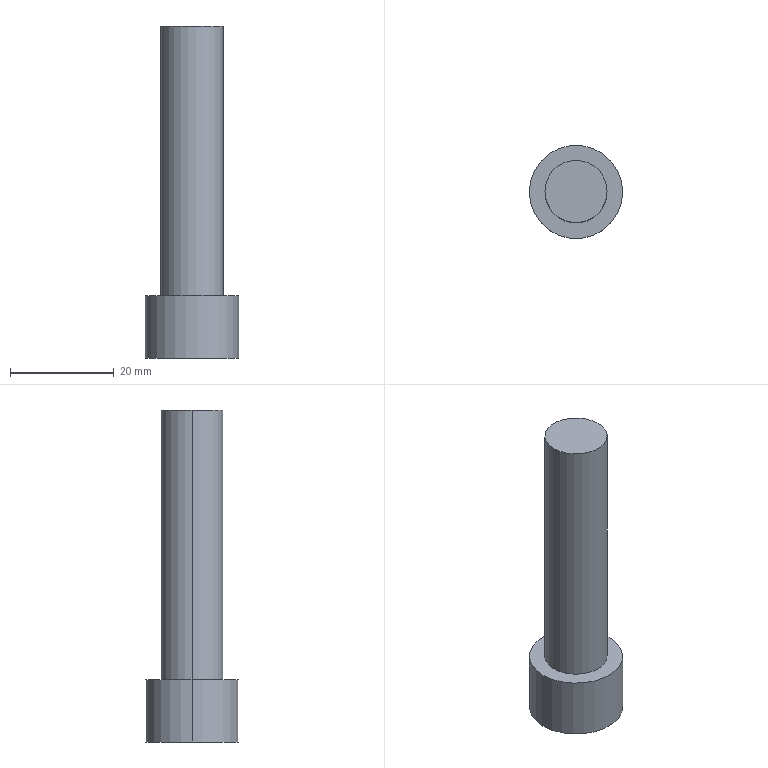Part | Creo | 1 solid | 14 faces | box 18 x 18 x 64 mm | volume 8415 mm3 | plane 10 | cylinder 4 | commonest cylinder face diameters 12 x2 18 x2
STEP:
#1=CARTESIAN_POINT('',(189.,0.,-294.5));
#2=VERTEX_POINT('',#1);
#3=CARTESIAN_POINT('',(171.,0.,-294.5));
#4=VERTEX_POINT('',#3);
#5=CARTESIAN_POINT('',(180.,0.,-294.5));
#6=DIRECTION('',(0.,0.,-1.));
#7=DIRECTION('',(1.,0.,0.));
#8=AXIS2_PLACEMENT_3D('',#5,#6,#7);
#9=CIRCLE('',#8,9.);
#10=EDGE_CURVE('',#2,#4,#9,.T.);
#11=ORIENTED_EDGE('',*,*,#10,.F.);
#12=CARTESIAN_POINT('',(180.,0.,-294.5));
#13=DIRECTION('',(0.,0.,-1.));
#14=DIRECTION('',(-1.,0.,0.));
#15=AXIS2_PLACEMENT_3D('',#12,#13,#14);
#16=CIRCLE('',#15,9.);
#17=EDGE_CURVE('',#4,#2,#16,.T.);
#18=ORIENTED_EDGE('',*,*,#17,.F.);
#19=EDGE_LOOP('',(#11,#18));
#20=FACE_OUTER_BOUND('',#19,.F.);
#21=CARTESIAN_POINT('',(175.,-2.887,-294.5));
#22=VERTEX_POINT('',#21);
#23=CARTESIAN_POINT('',(180.,-5.774,-294.5));
#24=VERTEX_POINT('',#23);
#25=CARTESIAN_POINT('',(175.,-2.887,-294.5));
#26=DIRECTION('',(0.866,-0.5,0.));
#27=VECTOR('',#26,5.774);
#28=LINE('',#25,#27);
#29=EDGE_CURVE('',#22,#24,#28,.T.);
#30=ORIENTED_EDGE('',*,*,#29,.F.);
#31=CARTESIAN_POINT('',(175.,2.887,-294.5));
#32=VERTEX_POINT('',#31);
#33=CARTESIAN_POINT('',(175.,-2.887,-294.5));
#34=DIRECTION('',(0.,1.,0.));
#35=VECTOR('',#34,5.774);
#36=LINE('',#33,#35);
#37=EDGE_CURVE('',#22,#32,#36,.T.);
#38=ORIENTED_EDGE('',*,*,#37,.T.);
#39=CARTESIAN_POINT('',(180.,5.774,-294.5));
#40=VERTEX_POINT('',#39);
#41=CARTESIAN_POINT('',(180.,5.774,-294.5));
#42=DIRECTION('',(-0.866,-0.5,0.));
#43=VECTOR('',#42,5.774);
#44=LINE('',#41,#43);
#45=EDGE_CURVE('',#40,#32,#44,.T.);
#46=ORIENTED_EDGE('',*,*,#45,.F.);
#47=CARTESIAN_POINT('',(185.,2.887,-294.5));
#48=VERTEX_POINT('',#47);
#49=CARTESIAN_POINT('',(185.,2.887,-294.5));
#50=DIRECTION('',(-0.866,0.5,0.));
#51=VECTOR('',#50,5.774);
#52=LINE('',#49,#51);
#53=EDGE_CURVE('',#48,#40,#52,.T.);
#54=ORIENTED_EDGE('',*,*,#53,.F.);
#55=CARTESIAN_POINT('',(185.,-2.887,-294.5));
#56=VERTEX_POINT('',#55);
#57=CARTESIAN_POINT('',(185.,2.887,-294.5));
#58=DIRECTION('',(0.,-1.,0.));
#59=VECTOR('',#58,5.774);
#60=LINE('',#57,#59);
#61=EDGE_CURVE('',#48,#56,#60,.T.);
#62=ORIENTED_EDGE('',*,*,#61,.T.);
#63=CARTESIAN_POINT('',(180.,-5.774,-294.5));
#64=DIRECTION('',(0.866,0.5,0.));
#65=VECTOR('',#64,5.774);
#66=LINE('',#63,#65);
#67=EDGE_CURVE('',#24,#56,#66,.T.);
#68=ORIENTED_EDGE('',*,*,#67,.F.);
#69=EDGE_LOOP('',(#30,#38,#46,#54,#62,#68));
#70=FACE_BOUND('',#69,.F.);
#71=CARTESIAN_POINT('',(180.,0.,-294.5));
#72=DIRECTION('',(0.,0.,-1.));
#73=DIRECTION('',(-1.,0.,0.));
#74=AXIS2_PLACEMENT_3D('',#71,#72,#73);
#75=PLANE('',#74);
#76=ADVANCED_FACE('',(#20,#70),#75,.T.);
#77=CARTESIAN_POINT('',(171.,0.,-282.5));
#78=VERTEX_POINT('',#77);
#79=CARTESIAN_POINT('',(189.,0.,-282.5));
#80=VERTEX_POINT('',#79);
#81=CARTESIAN_POINT('',(180.,0.,-282.5));
#82=DIRECTION('',(0.,0.,1.));
#83=DIRECTION('',(-1.,0.,0.));
#84=AXIS2_PLACEMENT_3D('',#81,#82,#83);
#85=CIRCLE('',#84,9.);
#86=EDGE_CURVE('',#78,#80,#85,.T.);
#87=ORIENTED_EDGE('',*,*,#86,.T.);
#88=CARTESIAN_POINT('',(189.,0.,-294.5));
#89=DIRECTION('',(0.,0.,1.));
#90=VECTOR('',#89,12.);
#91=LINE('',#88,#90);
#92=EDGE_CURVE('',#2,#80,#91,.T.);
#93=ORIENTED_EDGE('',*,*,#92,.F.);
#94=ORIENTED_EDGE('',*,*,#10,.T.);
#95=CARTESIAN_POINT('',(171.,0.,-294.5));
#96=DIRECTION('',(0.,0.,1.));
#97=VECTOR('',#96,12.);
#98=LINE('',#95,#97);
#99=EDGE_CURVE('',#4,#78,#98,.T.);
#100=ORIENTED_EDGE('',*,*,#99,.T.);
#101=EDGE_LOOP('',(#87,#93,#94,#100));
#102=FACE_OUTER_BOUND('',#101,.F.);
#103=CARTESIAN_POINT('',(180.,0.,-294.5));
#104=DIRECTION('',(0.,0.,1.));
#105=DIRECTION('',(1.,0.,0.));
#106=AXIS2_PLACEMENT_3D('',#103,#104,#105);
#107=CYLINDRICAL_SURFACE('',#106,9.);
#108=ADVANCED_FACE('',(#102),#107,.T.);
#109=ORIENTED_EDGE('',*,*,#86,.F.);
#110=CARTESIAN_POINT('',(180.,0.,-282.5));
#111=DIRECTION('',(0.,0.,1.));
#112=DIRECTION('',(1.,0.,0.));
#113=AXIS2_PLACEMENT_3D('',#110,#111,#112);
#114=CIRCLE('',#113,9.);
#115=EDGE_CURVE('',#80,#78,#114,.T.);
#116=ORIENTED_EDGE('',*,*,#115,.F.);
#117=EDGE_LOOP('',(#109,#116));
#118=FACE_OUTER_BOUND('',#117,.F.);
#119=CARTESIAN_POINT('',(186.,0.,-282.5));
#120=VERTEX_POINT('',#119);
#121=CARTESIAN_POINT('',(174.,0.,-282.5));
#122=VERTEX_POINT('',#121);
#123=CARTESIAN_POINT('',(180.,0.,-282.5));
#124=DIRECTION('',(0.,0.,-1.));
#125=DIRECTION('',(1.,0.,0.));
#126=AXIS2_PLACEMENT_3D('',#123,#124,#125);
#127=CIRCLE('',#126,6.);
#128=EDGE_CURVE('',#120,#122,#127,.T.);
#129=ORIENTED_EDGE('',*,*,#128,.F.);
#130=CARTESIAN_POINT('',(180.,0.,-282.5));
#131=DIRECTION('',(0.,0.,-1.));
#132=DIRECTION('',(-1.,0.,0.));
#133=AXIS2_PLACEMENT_3D('',#130,#131,#132);
#134=CIRCLE('',#133,6.);
#135=EDGE_CURVE('',#122,#120,#134,.T.);
#136=ORIENTED_EDGE('',*,*,#135,.F.);
#137=EDGE_LOOP('',(#129,#136));
#138=FACE_BOUND('',#137,.F.);
#139=CARTESIAN_POINT('',(180.,0.,-282.5));
#140=DIRECTION('',(0.,0.,1.));
#141=DIRECTION('',(1.,0.,0.));
#142=AXIS2_PLACEMENT_3D('',#139,#140,#141);
#143=PLANE('',#142);
#144=ADVANCED_FACE('',(#118,#138),#143,.T.);
#145=ORIENTED_EDGE('',*,*,#128,.T.);
#146=CARTESIAN_POINT('',(174.,0.,-230.5));
#147=VERTEX_POINT('',#146);
#148=CARTESIAN_POINT('',(174.,0.,-282.5));
#149=DIRECTION('',(0.,0.,1.));
#150=VECTOR('',#149,52.);
#151=LINE('',#148,#150);
#152=EDGE_CURVE('',#122,#147,#151,.T.);
#153=ORIENTED_EDGE('',*,*,#152,.T.);
#154=CARTESIAN_POINT('',(186.,0.,-230.5));
#155=VERTEX_POINT('',#154);
#156=CARTESIAN_POINT('',(180.,0.,-230.5));
#157=DIRECTION('',(0.,0.,1.));
#158=DIRECTION('',(-1.,0.,0.));
#159=AXIS2_PLACEMENT_3D('',#156,#157,#158);
#160=CIRCLE('',#159,6.);
#161=EDGE_CURVE('',#147,#155,#160,.T.);
#162=ORIENTED_EDGE('',*,*,#161,.T.);
#163=CARTESIAN_POINT('',(186.,0.,-282.5));
#164=DIRECTION('',(0.,0.,1.));
#165=VECTOR('',#164,52.);
#166=LINE('',#163,#165);
#167=EDGE_CURVE('',#120,#155,#166,.T.);
#168=ORIENTED_EDGE('',*,*,#167,.F.);
#169=EDGE_LOOP('',(#145,#153,#162,#168));
#170=FACE_OUTER_BOUND('',#169,.F.);
#171=CARTESIAN_POINT('',(180.,0.,-284.5));
#172=DIRECTION('',(0.,0.,1.));
#173=DIRECTION('',(1.,0.,0.));
#174=AXIS2_PLACEMENT_3D('',#171,#172,#173);
#175=CYLINDRICAL_SURFACE('',#174,6.);
#176=ADVANCED_FACE('',(#170),#175,.T.);
#177=ORIENTED_EDGE('',*,*,#135,.T.);
#178=ORIENTED_EDGE('',*,*,#167,.T.);
#179=CARTESIAN_POINT('',(180.,0.,-230.5));
#180=DIRECTION('',(0.,0.,1.));
#181=DIRECTION('',(1.,0.,0.));
#182=AXIS2_PLACEMENT_3D('',#179,#180,#181);
#183=CIRCLE('',#182,6.);
#184=EDGE_CURVE('',#155,#147,#183,.T.);
#185=ORIENTED_EDGE('',*,*,#184,.T.);
#186=ORIENTED_EDGE('',*,*,#152,.F.);
#187=EDGE_LOOP('',(#177,#178,#185,#186));
#188=FACE_OUTER_BOUND('',#187,.F.);
#189=CARTESIAN_POINT('',(180.,0.,-284.5));
#190=DIRECTION('',(0.,0.,1.));
#191=DIRECTION('',(1.,0.,0.));
#192=AXIS2_PLACEMENT_3D('',#189,#190,#191);
#193=CYLINDRICAL_SURFACE('',#192,6.);
#194=ADVANCED_FACE('',(#188),#193,.T.);
#195=ORIENTED_EDGE('',*,*,#161,.F.);
#196=ORIENTED_EDGE('',*,*,#184,.F.);
#197=EDGE_LOOP('',(#195,#196));
#198=FACE_OUTER_BOUND('',#197,.F.);
#199=CARTESIAN_POINT('',(180.,0.,-230.5));
#200=DIRECTION('',(0.,0.,1.));
#201=DIRECTION('',(1.,0.,0.));
#202=AXIS2_PLACEMENT_3D('',#199,#200,#201);
#203=PLANE('',#202);
#204=ADVANCED_FACE('',(#198),#203,.T.);
#205=ORIENTED_EDGE('',*,*,#115,.T.);
#206=ORIENTED_EDGE('',*,*,#99,.F.);
#207=ORIENTED_EDGE('',*,*,#17,.T.);
#208=ORIENTED_EDGE('',*,*,#92,.T.);
#209=EDGE_LOOP('',(#205,#206,#207,#208));
#210=FACE_OUTER_BOUND('',#209,.F.);
#211=CARTESIAN_POINT('',(180.,0.,-294.5));
#212=DIRECTION('',(0.,0.,1.));
#213=DIRECTION('',(1.,0.,0.));
#214=AXIS2_PLACEMENT_3D('',#211,#212,#213);
#215=CYLINDRICAL_SURFACE('',#214,9.);
#216=ADVANCED_FACE('',(#210),#215,.T.);
#217=CARTESIAN_POINT('',(180.,-5.774,-288.5));
#218=VERTEX_POINT('',#217);
#219=CARTESIAN_POINT('',(175.,-2.887,-288.5));
#220=VERTEX_POINT('',#219);
#221=CARTESIAN_POINT('',(180.,-5.774,-288.5));
#222=DIRECTION('',(-0.866,0.5,0.));
#223=VECTOR('',#222,5.774);
#224=LINE('',#221,#223);
#225=EDGE_CURVE('',#218,#220,#224,.T.);
#226=ORIENTED_EDGE('',*,*,#225,.T.);
#227=CARTESIAN_POINT('',(175.,-2.887,-288.5));
#228=DIRECTION('',(0.,0.,-1.));
#229=VECTOR('',#228,6.);
#230=LINE('',#227,#229);
#231=EDGE_CURVE('',#220,#22,#230,.T.);
#232=ORIENTED_EDGE('',*,*,#231,.T.);
#233=ORIENTED_EDGE('',*,*,#29,.T.);
#234=CARTESIAN_POINT('',(180.,-5.774,-288.5));
#235=DIRECTION('',(0.,0.,-1.));
#236=VECTOR('',#235,6.);
#237=LINE('',#234,#236);
#238=EDGE_CURVE('',#218,#24,#237,.T.);
#239=ORIENTED_EDGE('',*,*,#238,.F.);
#240=EDGE_LOOP('',(#226,#232,#233,#239));
#241=FACE_OUTER_BOUND('',#240,.F.);
#242=CARTESIAN_POINT('',(177.5,-4.33,-291.5));
#243=DIRECTION('',(-0.5,-0.866,0.));
#244=DIRECTION('',(0.866,-0.5,0.));
#245=AXIS2_PLACEMENT_3D('',#242,#243,#244);
#246=PLANE('',#245);
#247=ADVANCED_FACE('',(#241),#246,.F.);
#248=CARTESIAN_POINT('',(175.,2.887,-288.5));
#249=VERTEX_POINT('',#248);
#250=CARTESIAN_POINT('',(175.,-2.887,-288.5));
#251=DIRECTION('',(0.,1.,0.));
#252=VECTOR('',#251,5.774);
#253=LINE('',#250,#252);
#254=EDGE_CURVE('',#220,#249,#253,.T.);
#255=ORIENTED_EDGE('',*,*,#254,.F.);
#256=ORIENTED_EDGE('',*,*,#225,.F.);
#257=CARTESIAN_POINT('',(185.,-2.887,-288.5));
#258=VERTEX_POINT('',#257);
#259=CARTESIAN_POINT('',(185.,-2.887,-288.5));
#260=DIRECTION('',(-0.866,-0.5,0.));
#261=VECTOR('',#260,5.774);
#262=LINE('',#259,#261);
#263=EDGE_CURVE('',#258,#218,#262,.T.);
#264=ORIENTED_EDGE('',*,*,#263,.F.);
#265=CARTESIAN_POINT('',(185.,2.887,-288.5));
#266=VERTEX_POINT('',#265);
#267=CARTESIAN_POINT('',(185.,2.887,-288.5));
#268=DIRECTION('',(0.,-1.,0.));
#269=VECTOR('',#268,5.774);
#270=LINE('',#267,#269);
#271=EDGE_CURVE('',#266,#258,#270,.T.);
#272=ORIENTED_EDGE('',*,*,#271,.F.);
#273=CARTESIAN_POINT('',(180.,5.774,-288.5));
#274=VERTEX_POINT('',#273);
#275=CARTESIAN_POINT('',(180.,5.774,-288.5));
#276=DIRECTION('',(0.866,-0.5,0.));
#277=VECTOR('',#276,5.774);
#278=LINE('',#275,#277);
#279=EDGE_CURVE('',#274,#266,#278,.T.);
#280=ORIENTED_EDGE('',*,*,#279,.F.);
#281=CARTESIAN_POINT('',(175.,2.887,-288.5));
#282=DIRECTION('',(0.866,0.5,0.));
#283=VECTOR('',#282,5.774);
#284=LINE('',#281,#283);
#285=EDGE_CURVE('',#249,#274,#284,.T.);
#286=ORIENTED_EDGE('',*,*,#285,.F.);
#287=EDGE_LOOP('',(#255,#256,#264,#272,#280,#286));
#288=FACE_OUTER_BOUND('',#287,.F.);
#289=CARTESIAN_POINT('',(180.,0.,-288.5));
#290=DIRECTION('',(0.,0.,1.));
#291=DIRECTION('',(1.,0.,0.));
#292=AXIS2_PLACEMENT_3D('',#289,#290,#291);
#293=PLANE('',#292);
#294=ADVANCED_FACE('',(#288),#293,.F.);
#295=ORIENTED_EDGE('',*,*,#254,.T.);
#296=CARTESIAN_POINT('',(175.,2.887,-288.5));
#297=DIRECTION('',(0.,0.,-1.));
#298=VECTOR('',#297,6.);
#299=LINE('',#296,#298);
#300=EDGE_CURVE('',#249,#32,#299,.T.);
#301=ORIENTED_EDGE('',*,*,#300,.T.);
#302=ORIENTED_EDGE('',*,*,#37,.F.);
#303=ORIENTED_EDGE('',*,*,#231,.F.);
#304=EDGE_LOOP('',(#295,#301,#302,#303));
#305=FACE_OUTER_BOUND('',#304,.F.);
#306=CARTESIAN_POINT('',(175.,0.,-291.5));
#307=DIRECTION('',(-1.,0.,0.));
#308=DIRECTION('',(0.,0.,1.));
#309=AXIS2_PLACEMENT_3D('',#306,#307,#308);
#310=PLANE('',#309);
#311=ADVANCED_FACE('',(#305),#310,.F.);
#312=ORIENTED_EDGE('',*,*,#285,.T.);
#313=CARTESIAN_POINT('',(180.,5.774,-288.5));
#314=DIRECTION('',(0.,0.,-1.));
#315=VECTOR('',#314,6.);
#316=LINE('',#313,#315);
#317=EDGE_CURVE('',#274,#40,#316,.T.);
#318=ORIENTED_EDGE('',*,*,#317,.T.);
#319=ORIENTED_EDGE('',*,*,#45,.T.);
#320=ORIENTED_EDGE('',*,*,#300,.F.);
#321=EDGE_LOOP('',(#312,#318,#319,#320));
#322=FACE_OUTER_BOUND('',#321,.F.);
#323=CARTESIAN_POINT('',(177.5,4.33,-291.5));
#324=DIRECTION('',(-0.5,0.866,0.));
#325=DIRECTION('',(-0.866,-0.5,0.));
#326=AXIS2_PLACEMENT_3D('',#323,#324,#325);
#327=PLANE('',#326);
#328=ADVANCED_FACE('',(#322),#327,.F.);
#329=ORIENTED_EDGE('',*,*,#279,.T.);
#330=CARTESIAN_POINT('',(185.,2.887,-288.5));
#331=DIRECTION('',(0.,0.,-1.));
#332=VECTOR('',#331,6.);
#333=LINE('',#330,#332);
#334=EDGE_CURVE('',#266,#48,#333,.T.);
#335=ORIENTED_EDGE('',*,*,#334,.T.);
#336=ORIENTED_EDGE('',*,*,#53,.T.);
#337=ORIENTED_EDGE('',*,*,#317,.F.);
#338=EDGE_LOOP('',(#329,#335,#336,#337));
#339=FACE_OUTER_BOUND('',#338,.F.);
#340=CARTESIAN_POINT('',(182.5,4.33,-291.5));
#341=DIRECTION('',(0.5,0.866,0.));
#342=DIRECTION('',(-0.866,0.5,0.));
#343=AXIS2_PLACEMENT_3D('',#340,#341,#342);
#344=PLANE('',#343);
#345=ADVANCED_FACE('',(#339),#344,.F.);
#346=ORIENTED_EDGE('',*,*,#271,.T.);
#347=CARTESIAN_POINT('',(185.,-2.887,-288.5));
#348=DIRECTION('',(0.,0.,-1.));
#349=VECTOR('',#348,6.);
#350=LINE('',#347,#349);
#351=EDGE_CURVE('',#258,#56,#350,.T.);
#352=ORIENTED_EDGE('',*,*,#351,.T.);
#353=ORIENTED_EDGE('',*,*,#61,.F.);
#354=ORIENTED_EDGE('',*,*,#334,.F.);
#355=EDGE_LOOP('',(#346,#352,#353,#354));
#356=FACE_OUTER_BOUND('',#355,.F.);
#357=CARTESIAN_POINT('',(185.,0.,-291.5));
#358=DIRECTION('',(1.,0.,0.));
#359=DIRECTION('',(0.,0.,-1.));
#360=AXIS2_PLACEMENT_3D('',#357,#358,#359);
#361=PLANE('',#360);
#362=ADVANCED_FACE('',(#356),#361,.F.);
#363=ORIENTED_EDGE('',*,*,#263,.T.);
#364=ORIENTED_EDGE('',*,*,#238,.T.);
#365=ORIENTED_EDGE('',*,*,#67,.T.);
#366=ORIENTED_EDGE('',*,*,#351,.F.);
#367=EDGE_LOOP('',(#363,#364,#365,#366));
#368=FACE_OUTER_BOUND('',#367,.F.);
#369=CARTESIAN_POINT('',(182.5,-4.33,-291.5));
#370=DIRECTION('',(0.5,-0.866,0.));
#371=DIRECTION('',(0.866,0.5,0.));
#372=AXIS2_PLACEMENT_3D('',#369,#370,#371);
#373=PLANE('',#372);
#374=ADVANCED_FACE('',(#368),#373,.F.);
#375=CLOSED_SHELL('',(#76,#108,#144,#176,#194,#204,#216,#247,#294,#311,#328,#345,#362,#374));
#376=MANIFOLD_SOLID_BREP('',#375);
#377=(LENGTH_UNIT()NAMED_UNIT(*)SI_UNIT(.MILLI.,.METRE.));
#378=UNCERTAINTY_MEASURE_WITH_UNIT(LENGTH_MEASURE(0.006887),#377,'','');
#379=(NAMED_UNIT(*)PLANE_ANGLE_UNIT()SI_UNIT($,.RADIAN.));
#380=PLANE_ANGLE_MEASURE_WITH_UNIT(PLANE_ANGLE_MEASURE(0.01745),#379);
#381=(CONVERSION_BASED_UNIT('DEGREE',#380)NAMED_UNIT(*)PLANE_ANGLE_UNIT());
#382=(NAMED_UNIT(*)SI_UNIT($,.STERADIAN.)SOLID_ANGLE_UNIT());
#383=(GEOMETRIC_REPRESENTATION_CONTEXT(3)GLOBAL_UNCERTAINTY_ASSIGNED_CONTEXT((#378))GLOBAL_UNIT_ASSIGNED_CONTEXT((#377,#381,#382))REPRESENTATION_CONTEXT('',''));
#384=ADVANCED_BREP_SHAPE_REPRESENTATION('',(#376),#383);